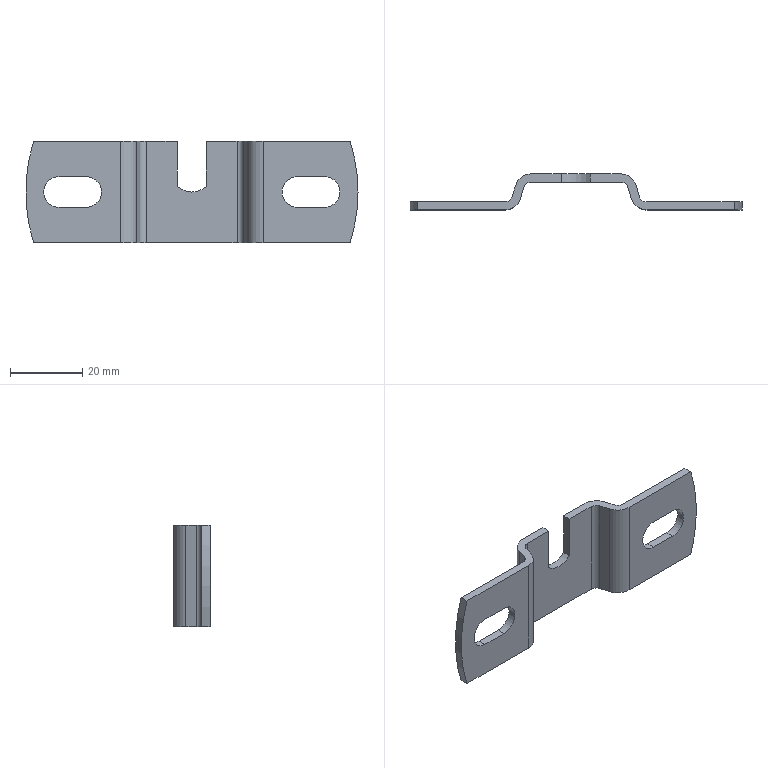Part | STEP file | ROLLER.HOLER.stp | 1 solid | 37 faces | box 92 x 10 x 28 mm | volume 5564 mm3 | plane 19 | cylinder 18 | commonest cylinder face diameters 8.5 x6 4 x4 9.2 x4 92 x3 12 x1